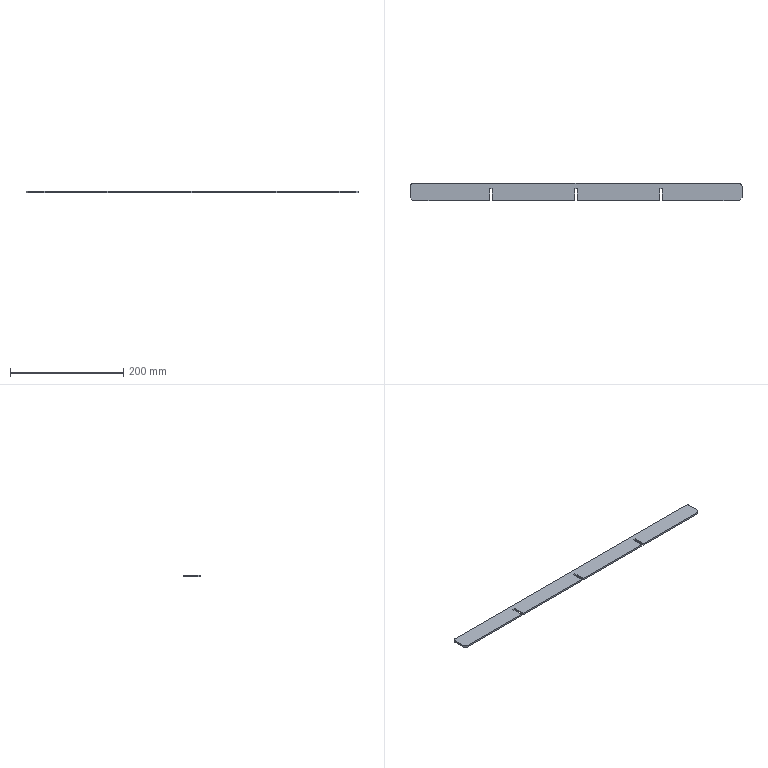Part | SolidWorks | features FlatPattern 1, SMBaseFlange 1, SheetMetal 1 | 1 solid | 22 faces | box 585.4 x 30 x 3 mm | volume 51728 mm3 | plane 20 | cylinder 2 | commonest cylinder face diameters 10 x2
STEP:
#1=CARTESIAN_POINT('',(-293.386,-592.7,0.));
#2=VERTEX_POINT('',#1);
#3=CARTESIAN_POINT('',(-288.386,-597.7,0.));
#4=VERTEX_POINT('',#3);
#5=CARTESIAN_POINT('',(-293.386,-592.7,0.));
#6=DIRECTION('',(0.7071,-0.7071,0.));
#7=VECTOR('',#6,1000.);
#8=LINE('',#5,#7);
#9=EDGE_CURVE('',#2,#4,#8,.T.);
#10=ORIENTED_EDGE('',*,*,#9,.F.);
#11=CARTESIAN_POINT('',(-293.386,-592.7,-3.));
#12=VERTEX_POINT('',#11);
#13=CARTESIAN_POINT('',(-293.386,-592.7,-3.));
#14=DIRECTION('',(0.,0.,1.));
#15=VECTOR('',#14,1000.);
#16=LINE('',#13,#15);
#17=EDGE_CURVE('',#12,#2,#16,.T.);
#18=ORIENTED_EDGE('',*,*,#17,.F.);
#19=CARTESIAN_POINT('',(-288.386,-597.7,-3.));
#20=VERTEX_POINT('',#19);
#21=CARTESIAN_POINT('',(-293.386,-592.7,-3.));
#22=DIRECTION('',(0.7071,-0.7071,0.));
#23=VECTOR('',#22,1000.);
#24=LINE('',#21,#23);
#25=EDGE_CURVE('',#12,#20,#24,.T.);
#26=ORIENTED_EDGE('',*,*,#25,.T.);
#27=CARTESIAN_POINT('',(-288.386,-597.7,-3.));
#28=DIRECTION('',(0.,0.,1.));
#29=VECTOR('',#28,1000.);
#30=LINE('',#27,#29);
#31=EDGE_CURVE('',#20,#4,#30,.T.);
#32=ORIENTED_EDGE('',*,*,#31,.T.);
#33=EDGE_LOOP('',(#10,#18,#26,#32));
#34=FACE_OUTER_BOUND('',#33,.T.);
#35=CARTESIAN_POINT('',(-293.386,-592.7,-3.));
#36=DIRECTION('',(-0.7071,-0.7071,0.));
#37=DIRECTION('',(0.7071,-0.7071,0.));
#38=AXIS2_PLACEMENT_3D('',#35,#36,#37);
#39=PLANE('',#38);
#40=ADVANCED_FACE('',(#34),#39,.T.);
#41=CARTESIAN_POINT('',(-293.386,-572.7,0.));
#42=VERTEX_POINT('',#41);
#43=CARTESIAN_POINT('',(-293.386,-572.7,0.));
#44=DIRECTION('',(0.,-1.,0.));
#45=VECTOR('',#44,1000.);
#46=LINE('',#43,#45);
#47=EDGE_CURVE('',#42,#2,#46,.T.);
#48=ORIENTED_EDGE('',*,*,#47,.F.);
#49=CARTESIAN_POINT('',(-293.386,-572.7,-3.));
#50=VERTEX_POINT('',#49);
#51=CARTESIAN_POINT('',(-293.386,-572.7,-3.));
#52=DIRECTION('',(0.,0.,1.));
#53=VECTOR('',#52,1000.);
#54=LINE('',#51,#53);
#55=EDGE_CURVE('',#50,#42,#54,.T.);
#56=ORIENTED_EDGE('',*,*,#55,.F.);
#57=CARTESIAN_POINT('',(-293.386,-572.7,-3.));
#58=DIRECTION('',(0.,-1.,0.));
#59=VECTOR('',#58,1000.);
#60=LINE('',#57,#59);
#61=EDGE_CURVE('',#50,#12,#60,.T.);
#62=ORIENTED_EDGE('',*,*,#61,.T.);
#63=ORIENTED_EDGE('',*,*,#17,.T.);
#64=EDGE_LOOP('',(#48,#56,#62,#63));
#65=FACE_OUTER_BOUND('',#64,.T.);
#66=CARTESIAN_POINT('',(-293.386,-572.7,-3.));
#67=DIRECTION('',(-1.,0.,0.));
#68=DIRECTION('',(0.,0.,1.));
#69=AXIS2_PLACEMENT_3D('',#66,#67,#68);
#70=PLANE('',#69);
#71=ADVANCED_FACE('',(#65),#70,.T.);
#72=CARTESIAN_POINT('',(-288.386,-567.7,0.));
#73=VERTEX_POINT('',#72);
#74=CARTESIAN_POINT('',(-288.386,-572.7,0.));
#75=DIRECTION('',(0.,0.,1.));
#76=DIRECTION('',(1.,0.,0.));
#77=AXIS2_PLACEMENT_3D('',#74,#75,#76);
#78=CIRCLE('',#77,5.);
#79=EDGE_CURVE('',#73,#42,#78,.T.);
#80=ORIENTED_EDGE('',*,*,#79,.F.);
#81=CARTESIAN_POINT('',(-288.386,-567.7,-3.));
#82=VERTEX_POINT('',#81);
#83=CARTESIAN_POINT('',(-288.386,-567.7,-3.));
#84=DIRECTION('',(0.,0.,1.));
#85=VECTOR('',#84,1000.);
#86=LINE('',#83,#85);
#87=EDGE_CURVE('',#82,#73,#86,.T.);
#88=ORIENTED_EDGE('',*,*,#87,.F.);
#89=CARTESIAN_POINT('',(-288.386,-572.7,-3.));
#90=DIRECTION('',(0.,0.,1.));
#91=DIRECTION('',(1.,0.,0.));
#92=AXIS2_PLACEMENT_3D('',#89,#90,#91);
#93=CIRCLE('',#92,5.);
#94=EDGE_CURVE('',#82,#50,#93,.T.);
#95=ORIENTED_EDGE('',*,*,#94,.T.);
#96=ORIENTED_EDGE('',*,*,#55,.T.);
#97=EDGE_LOOP('',(#80,#88,#95,#96));
#98=FACE_OUTER_BOUND('',#97,.T.);
#99=CARTESIAN_POINT('',(-288.386,-572.7,-3.));
#100=DIRECTION('',(0.,0.,1.));
#101=DIRECTION('',(1.,0.,0.));
#102=AXIS2_PLACEMENT_3D('',#99,#100,#101);
#103=CYLINDRICAL_SURFACE('',#102,5.);
#104=ADVANCED_FACE('',(#98),#103,.T.);
#105=CARTESIAN_POINT('',(287.014,-567.7,0.));
#106=VERTEX_POINT('',#105);
#107=CARTESIAN_POINT('',(287.014,-567.7,0.));
#108=DIRECTION('',(-1.,0.,0.));
#109=VECTOR('',#108,1000.);
#110=LINE('',#107,#109);
#111=EDGE_CURVE('',#106,#73,#110,.T.);
#112=ORIENTED_EDGE('',*,*,#111,.F.);
#113=CARTESIAN_POINT('',(287.014,-567.7,-3.));
#114=VERTEX_POINT('',#113);
#115=CARTESIAN_POINT('',(287.014,-567.7,-3.));
#116=DIRECTION('',(0.,0.,1.));
#117=VECTOR('',#116,1000.);
#118=LINE('',#115,#117);
#119=EDGE_CURVE('',#114,#106,#118,.T.);
#120=ORIENTED_EDGE('',*,*,#119,.F.);
#121=CARTESIAN_POINT('',(287.014,-567.7,-3.));
#122=DIRECTION('',(-1.,0.,0.));
#123=VECTOR('',#122,1000.);
#124=LINE('',#121,#123);
#125=EDGE_CURVE('',#114,#82,#124,.T.);
#126=ORIENTED_EDGE('',*,*,#125,.T.);
#127=ORIENTED_EDGE('',*,*,#87,.T.);
#128=EDGE_LOOP('',(#112,#120,#126,#127));
#129=FACE_OUTER_BOUND('',#128,.T.);
#130=CARTESIAN_POINT('',(287.014,-567.7,-3.));
#131=DIRECTION('',(0.,1.,0.));
#132=DIRECTION('',(-1.,0.,0.));
#133=AXIS2_PLACEMENT_3D('',#130,#131,#132);
#134=PLANE('',#133);
#135=ADVANCED_FACE('',(#129),#134,.T.);
#136=CARTESIAN_POINT('',(292.014,-572.7,0.));
#137=VERTEX_POINT('',#136);
#138=CARTESIAN_POINT('',(287.014,-572.7,0.));
#139=DIRECTION('',(0.,0.,1.));
#140=DIRECTION('',(-1.,0.,0.));
#141=AXIS2_PLACEMENT_3D('',#138,#139,#140);
#142=CIRCLE('',#141,5.);
#143=EDGE_CURVE('',#137,#106,#142,.T.);
#144=ORIENTED_EDGE('',*,*,#143,.F.);
#145=CARTESIAN_POINT('',(292.014,-572.7,-3.));
#146=VERTEX_POINT('',#145);
#147=CARTESIAN_POINT('',(292.014,-572.7,-3.));
#148=DIRECTION('',(0.,0.,1.));
#149=VECTOR('',#148,1000.);
#150=LINE('',#147,#149);
#151=EDGE_CURVE('',#146,#137,#150,.T.);
#152=ORIENTED_EDGE('',*,*,#151,.F.);
#153=CARTESIAN_POINT('',(287.014,-572.7,-3.));
#154=DIRECTION('',(0.,0.,1.));
#155=DIRECTION('',(-1.,0.,0.));
#156=AXIS2_PLACEMENT_3D('',#153,#154,#155);
#157=CIRCLE('',#156,5.);
#158=EDGE_CURVE('',#146,#114,#157,.T.);
#159=ORIENTED_EDGE('',*,*,#158,.T.);
#160=ORIENTED_EDGE('',*,*,#119,.T.);
#161=EDGE_LOOP('',(#144,#152,#159,#160));
#162=FACE_OUTER_BOUND('',#161,.T.);
#163=CARTESIAN_POINT('',(287.014,-572.7,-3.));
#164=DIRECTION('',(0.,0.,1.));
#165=DIRECTION('',(1.,0.,0.));
#166=AXIS2_PLACEMENT_3D('',#163,#164,#165);
#167=CYLINDRICAL_SURFACE('',#166,5.);
#168=ADVANCED_FACE('',(#162),#167,.T.);
#169=CARTESIAN_POINT('',(292.014,-592.7,0.));
#170=VERTEX_POINT('',#169);
#171=CARTESIAN_POINT('',(292.014,-592.7,0.));
#172=DIRECTION('',(0.,1.,0.));
#173=VECTOR('',#172,1000.);
#174=LINE('',#171,#173);
#175=EDGE_CURVE('',#170,#137,#174,.T.);
#176=ORIENTED_EDGE('',*,*,#175,.F.);
#177=CARTESIAN_POINT('',(292.014,-592.7,-3.));
#178=VERTEX_POINT('',#177);
#179=CARTESIAN_POINT('',(292.014,-592.7,-3.));
#180=DIRECTION('',(0.,0.,1.));
#181=VECTOR('',#180,1000.);
#182=LINE('',#179,#181);
#183=EDGE_CURVE('',#178,#170,#182,.T.);
#184=ORIENTED_EDGE('',*,*,#183,.F.);
#185=CARTESIAN_POINT('',(292.014,-592.7,-3.));
#186=DIRECTION('',(0.,1.,0.));
#187=VECTOR('',#186,1000.);
#188=LINE('',#185,#187);
#189=EDGE_CURVE('',#178,#146,#188,.T.);
#190=ORIENTED_EDGE('',*,*,#189,.T.);
#191=ORIENTED_EDGE('',*,*,#151,.T.);
#192=EDGE_LOOP('',(#176,#184,#190,#191));
#193=FACE_OUTER_BOUND('',#192,.T.);
#194=CARTESIAN_POINT('',(292.014,-592.7,-3.));
#195=DIRECTION('',(1.,0.,0.));
#196=DIRECTION('',(0.,0.,-1.));
#197=AXIS2_PLACEMENT_3D('',#194,#195,#196);
#198=PLANE('',#197);
#199=ADVANCED_FACE('',(#193),#198,.T.);
#200=CARTESIAN_POINT('',(287.014,-597.7,0.));
#201=VERTEX_POINT('',#200);
#202=CARTESIAN_POINT('',(287.014,-597.7,0.));
#203=DIRECTION('',(0.7071,0.7071,0.));
#204=VECTOR('',#203,1000.);
#205=LINE('',#202,#204);
#206=EDGE_CURVE('',#201,#170,#205,.T.);
#207=ORIENTED_EDGE('',*,*,#206,.F.);
#208=CARTESIAN_POINT('',(287.014,-597.7,-3.));
#209=VERTEX_POINT('',#208);
#210=CARTESIAN_POINT('',(287.014,-597.7,-3.));
#211=DIRECTION('',(0.,0.,1.));
#212=VECTOR('',#211,1000.);
#213=LINE('',#210,#212);
#214=EDGE_CURVE('',#209,#201,#213,.T.);
#215=ORIENTED_EDGE('',*,*,#214,.F.);
#216=CARTESIAN_POINT('',(287.014,-597.7,-3.));
#217=DIRECTION('',(0.7071,0.7071,0.));
#218=VECTOR('',#217,1000.);
#219=LINE('',#216,#218);
#220=EDGE_CURVE('',#209,#178,#219,.T.);
#221=ORIENTED_EDGE('',*,*,#220,.T.);
#222=ORIENTED_EDGE('',*,*,#183,.T.);
#223=EDGE_LOOP('',(#207,#215,#221,#222));
#224=FACE_OUTER_BOUND('',#223,.T.);
#225=CARTESIAN_POINT('',(287.014,-597.7,-3.));
#226=DIRECTION('',(0.7071,-0.7071,0.));
#227=DIRECTION('',(0.7071,0.7071,0.));
#228=AXIS2_PLACEMENT_3D('',#225,#226,#227);
#229=PLANE('',#228);
#230=ADVANCED_FACE('',(#224),#229,.T.);
#231=CARTESIAN_POINT('',(151.564,-597.7,0.));
#232=VERTEX_POINT('',#231);
#233=CARTESIAN_POINT('',(151.564,-597.7,0.));
#234=DIRECTION('',(1.,0.,0.));
#235=VECTOR('',#234,1000.);
#236=LINE('',#233,#235);
#237=EDGE_CURVE('',#232,#201,#236,.T.);
#238=ORIENTED_EDGE('',*,*,#237,.F.);
#239=CARTESIAN_POINT('',(151.564,-597.7,-3.));
#240=VERTEX_POINT('',#239);
#241=CARTESIAN_POINT('',(151.564,-597.7,-3.));
#242=DIRECTION('',(0.,0.,1.));
#243=VECTOR('',#242,1000.);
#244=LINE('',#241,#243);
#245=EDGE_CURVE('',#240,#232,#244,.T.);
#246=ORIENTED_EDGE('',*,*,#245,.F.);
#247=CARTESIAN_POINT('',(151.564,-597.7,-3.));
#248=DIRECTION('',(1.,0.,0.));
#249=VECTOR('',#248,1000.);
#250=LINE('',#247,#249);
#251=EDGE_CURVE('',#240,#209,#250,.T.);
#252=ORIENTED_EDGE('',*,*,#251,.T.);
#253=ORIENTED_EDGE('',*,*,#214,.T.);
#254=EDGE_LOOP('',(#238,#246,#252,#253));
#255=FACE_OUTER_BOUND('',#254,.T.);
#256=CARTESIAN_POINT('',(151.564,-597.7,-3.));
#257=DIRECTION('',(0.,-1.,0.));
#258=DIRECTION('',(1.,0.,0.));
#259=AXIS2_PLACEMENT_3D('',#256,#257,#258);
#260=PLANE('',#259);
#261=ADVANCED_FACE('',(#255),#260,.T.);
#262=CARTESIAN_POINT('',(151.564,-576.7,0.));
#263=VERTEX_POINT('',#262);
#264=CARTESIAN_POINT('',(151.564,-576.7,0.));
#265=DIRECTION('',(0.,-1.,0.));
#266=VECTOR('',#265,1000.);
#267=LINE('',#264,#266);
#268=EDGE_CURVE('',#263,#232,#267,.T.);
#269=ORIENTED_EDGE('',*,*,#268,.F.);
#270=CARTESIAN_POINT('',(151.564,-576.7,-3.));
#271=VERTEX_POINT('',#270);
#272=CARTESIAN_POINT('',(151.564,-576.7,-3.));
#273=DIRECTION('',(0.,0.,1.));
#274=VECTOR('',#273,1000.);
#275=LINE('',#272,#274);
#276=EDGE_CURVE('',#271,#263,#275,.T.);
#277=ORIENTED_EDGE('',*,*,#276,.F.);
#278=CARTESIAN_POINT('',(151.564,-576.7,-3.));
#279=DIRECTION('',(0.,-1.,0.));
#280=VECTOR('',#279,1000.);
#281=LINE('',#278,#280);
#282=EDGE_CURVE('',#271,#240,#281,.T.);
#283=ORIENTED_EDGE('',*,*,#282,.T.);
#284=ORIENTED_EDGE('',*,*,#245,.T.);
#285=EDGE_LOOP('',(#269,#277,#283,#284));
#286=FACE_OUTER_BOUND('',#285,.T.);
#287=CARTESIAN_POINT('',(151.564,-576.7,-3.));
#288=DIRECTION('',(-1.,0.,0.));
#289=DIRECTION('',(0.,0.,1.));
#290=AXIS2_PLACEMENT_3D('',#287,#288,#289);
#291=PLANE('',#290);
#292=ADVANCED_FACE('',(#286),#291,.T.);
#293=CARTESIAN_POINT('',(147.064,-576.7,0.));
#294=VERTEX_POINT('',#293);
#295=CARTESIAN_POINT('',(147.064,-576.7,0.));
#296=DIRECTION('',(1.,0.,0.));
#297=VECTOR('',#296,1000.);
#298=LINE('',#295,#297);
#299=EDGE_CURVE('',#294,#263,#298,.T.);
#300=ORIENTED_EDGE('',*,*,#299,.F.);
#301=CARTESIAN_POINT('',(147.064,-576.7,-3.));
#302=VERTEX_POINT('',#301);
#303=CARTESIAN_POINT('',(147.064,-576.7,-3.));
#304=DIRECTION('',(0.,0.,1.));
#305=VECTOR('',#304,1000.);
#306=LINE('',#303,#305);
#307=EDGE_CURVE('',#302,#294,#306,.T.);
#308=ORIENTED_EDGE('',*,*,#307,.F.);
#309=CARTESIAN_POINT('',(147.064,-576.7,-3.));
#310=DIRECTION('',(1.,0.,0.));
#311=VECTOR('',#310,1000.);
#312=LINE('',#309,#311);
#313=EDGE_CURVE('',#302,#271,#312,.T.);
#314=ORIENTED_EDGE('',*,*,#313,.T.);
#315=ORIENTED_EDGE('',*,*,#276,.T.);
#316=EDGE_LOOP('',(#300,#308,#314,#315));
#317=FACE_OUTER_BOUND('',#316,.T.);
#318=CARTESIAN_POINT('',(147.064,-576.7,-3.));
#319=DIRECTION('',(0.,-1.,0.));
#320=DIRECTION('',(0.,0.,-1.));
#321=AXIS2_PLACEMENT_3D('',#318,#319,#320);
#322=PLANE('',#321);
#323=ADVANCED_FACE('',(#317),#322,.T.);
#324=CARTESIAN_POINT('',(147.064,-597.7,0.));
#325=VERTEX_POINT('',#324);
#326=CARTESIAN_POINT('',(147.064,-597.7,0.));
#327=DIRECTION('',(0.,1.,0.));
#328=VECTOR('',#327,1000.);
#329=LINE('',#326,#328);
#330=EDGE_CURVE('',#325,#294,#329,.T.);
#331=ORIENTED_EDGE('',*,*,#330,.F.);
#332=CARTESIAN_POINT('',(147.064,-597.7,-3.));
#333=VERTEX_POINT('',#332);
#334=CARTESIAN_POINT('',(147.064,-597.7,-3.));
#335=DIRECTION('',(0.,0.,1.));
#336=VECTOR('',#335,1000.);
#337=LINE('',#334,#336);
#338=EDGE_CURVE('',#333,#325,#337,.T.);
#339=ORIENTED_EDGE('',*,*,#338,.F.);
#340=CARTESIAN_POINT('',(147.064,-597.7,-3.));
#341=DIRECTION('',(0.,1.,0.));
#342=VECTOR('',#341,1000.);
#343=LINE('',#340,#342);
#344=EDGE_CURVE('',#333,#302,#343,.T.);
#345=ORIENTED_EDGE('',*,*,#344,.T.);
#346=ORIENTED_EDGE('',*,*,#307,.T.);
#347=EDGE_LOOP('',(#331,#339,#345,#346));
#348=FACE_OUTER_BOUND('',#347,.T.);
#349=CARTESIAN_POINT('',(147.064,-597.7,-3.));
#350=DIRECTION('',(1.,0.,0.));
#351=DIRECTION('',(0.,0.,-1.));
#352=AXIS2_PLACEMENT_3D('',#349,#350,#351);
#353=PLANE('',#352);
#354=ADVANCED_FACE('',(#348),#353,.T.);
#355=CARTESIAN_POINT('',(1.564,-597.7,0.));
#356=VERTEX_POINT('',#355);
#357=CARTESIAN_POINT('',(1.564,-597.7,0.));
#358=DIRECTION('',(1.,0.,0.));
#359=VECTOR('',#358,1000.);
#360=LINE('',#357,#359);
#361=EDGE_CURVE('',#356,#325,#360,.T.);
#362=ORIENTED_EDGE('',*,*,#361,.F.);
#363=CARTESIAN_POINT('',(1.564,-597.7,-3.));
#364=VERTEX_POINT('',#363);
#365=CARTESIAN_POINT('',(1.564,-597.7,-3.));
#366=DIRECTION('',(0.,0.,1.));
#367=VECTOR('',#366,1000.);
#368=LINE('',#365,#367);
#369=EDGE_CURVE('',#364,#356,#368,.T.);
#370=ORIENTED_EDGE('',*,*,#369,.F.);
#371=CARTESIAN_POINT('',(1.564,-597.7,-3.));
#372=DIRECTION('',(1.,0.,0.));
#373=VECTOR('',#372,1000.);
#374=LINE('',#371,#373);
#375=EDGE_CURVE('',#364,#333,#374,.T.);
#376=ORIENTED_EDGE('',*,*,#375,.T.);
#377=ORIENTED_EDGE('',*,*,#338,.T.);
#378=EDGE_LOOP('',(#362,#370,#376,#377));
#379=FACE_OUTER_BOUND('',#378,.T.);
#380=CARTESIAN_POINT('',(1.564,-597.7,-3.));
#381=DIRECTION('',(0.,-1.,0.));
#382=DIRECTION('',(1.,0.,0.));
#383=AXIS2_PLACEMENT_3D('',#380,#381,#382);
#384=PLANE('',#383);
#385=ADVANCED_FACE('',(#379),#384,.T.);
#386=CARTESIAN_POINT('',(1.564,-576.7,0.));
#387=VERTEX_POINT('',#386);
#388=CARTESIAN_POINT('',(1.564,-576.7,0.));
#389=DIRECTION('',(0.,-1.,0.));
#390=VECTOR('',#389,1000.);
#391=LINE('',#388,#390);
#392=EDGE_CURVE('',#387,#356,#391,.T.);
#393=ORIENTED_EDGE('',*,*,#392,.F.);
#394=CARTESIAN_POINT('',(1.564,-576.7,-3.));
#395=VERTEX_POINT('',#394);
#396=CARTESIAN_POINT('',(1.564,-576.7,-3.));
#397=DIRECTION('',(0.,0.,1.));
#398=VECTOR('',#397,1000.);
#399=LINE('',#396,#398);
#400=EDGE_CURVE('',#395,#387,#399,.T.);
#401=ORIENTED_EDGE('',*,*,#400,.F.);
#402=CARTESIAN_POINT('',(1.564,-576.7,-3.));
#403=DIRECTION('',(0.,-1.,0.));
#404=VECTOR('',#403,1000.);
#405=LINE('',#402,#404);
#406=EDGE_CURVE('',#395,#364,#405,.T.);
#407=ORIENTED_EDGE('',*,*,#406,.T.);
#408=ORIENTED_EDGE('',*,*,#369,.T.);
#409=EDGE_LOOP('',(#393,#401,#407,#408));
#410=FACE_OUTER_BOUND('',#409,.T.);
#411=CARTESIAN_POINT('',(1.564,-576.7,-3.));
#412=DIRECTION('',(-1.,0.,0.));
#413=DIRECTION('',(0.,-1.,0.));
#414=AXIS2_PLACEMENT_3D('',#411,#412,#413);
#415=PLANE('',#414);
#416=ADVANCED_FACE('',(#410),#415,.T.);
#417=CARTESIAN_POINT('',(-2.936,-576.7,0.));
#418=VERTEX_POINT('',#417);
#419=CARTESIAN_POINT('',(-2.936,-576.7,0.));
#420=DIRECTION('',(1.,0.,0.));
#421=VECTOR('',#420,1000.);
#422=LINE('',#419,#421);
#423=EDGE_CURVE('',#418,#387,#422,.T.);
#424=ORIENTED_EDGE('',*,*,#423,.F.);
#425=CARTESIAN_POINT('',(-2.936,-576.7,-3.));
#426=VERTEX_POINT('',#425);
#427=CARTESIAN_POINT('',(-2.936,-576.7,-3.));
#428=DIRECTION('',(0.,0.,1.));
#429=VECTOR('',#428,1000.);
#430=LINE('',#427,#429);
#431=EDGE_CURVE('',#426,#418,#430,.T.);
#432=ORIENTED_EDGE('',*,*,#431,.F.);
#433=CARTESIAN_POINT('',(-2.936,-576.7,-3.));
#434=DIRECTION('',(1.,0.,0.));
#435=VECTOR('',#434,1000.);
#436=LINE('',#433,#435);
#437=EDGE_CURVE('',#426,#395,#436,.T.);
#438=ORIENTED_EDGE('',*,*,#437,.T.);
#439=ORIENTED_EDGE('',*,*,#400,.T.);
#440=EDGE_LOOP('',(#424,#432,#438,#439));
#441=FACE_OUTER_BOUND('',#440,.T.);
#442=CARTESIAN_POINT('',(-2.936,-576.7,-3.));
#443=DIRECTION('',(0.,-1.,0.));
#444=DIRECTION('',(0.,0.,-1.));
#445=AXIS2_PLACEMENT_3D('',#442,#443,#444);
#446=PLANE('',#445);
#447=ADVANCED_FACE('',(#441),#446,.T.);
#448=CARTESIAN_POINT('',(-2.936,-597.7,0.));
#449=VERTEX_POINT('',#448);
#450=CARTESIAN_POINT('',(-2.936,-597.7,0.));
#451=DIRECTION('',(0.,1.,0.));
#452=VECTOR('',#451,1000.);
#453=LINE('',#450,#452);
#454=EDGE_CURVE('',#449,#418,#453,.T.);
#455=ORIENTED_EDGE('',*,*,#454,.F.);
#456=CARTESIAN_POINT('',(-2.936,-597.7,-3.));
#457=VERTEX_POINT('',#456);
#458=CARTESIAN_POINT('',(-2.936,-597.7,-3.));
#459=DIRECTION('',(0.,0.,1.));
#460=VECTOR('',#459,1000.);
#461=LINE('',#458,#460);
#462=EDGE_CURVE('',#457,#449,#461,.T.);
#463=ORIENTED_EDGE('',*,*,#462,.F.);
#464=CARTESIAN_POINT('',(-2.936,-597.7,-3.));
#465=DIRECTION('',(0.,1.,0.));
#466=VECTOR('',#465,1000.);
#467=LINE('',#464,#466);
#468=EDGE_CURVE('',#457,#426,#467,.T.);
#469=ORIENTED_EDGE('',*,*,#468,.T.);
#470=ORIENTED_EDGE('',*,*,#431,.T.);
#471=EDGE_LOOP('',(#455,#463,#469,#470));
#472=FACE_OUTER_BOUND('',#471,.T.);
#473=CARTESIAN_POINT('',(-2.936,-597.7,-3.));
#474=DIRECTION('',(1.,0.,0.));
#475=DIRECTION('',(0.,0.,-1.));
#476=AXIS2_PLACEMENT_3D('',#473,#474,#475);
#477=PLANE('',#476);
#478=ADVANCED_FACE('',(#472),#477,.T.);
#479=CARTESIAN_POINT('',(-148.436,-597.7,0.));
#480=VERTEX_POINT('',#479);
#481=CARTESIAN_POINT('',(-148.436,-597.7,0.));
#482=DIRECTION('',(1.,0.,0.));
#483=VECTOR('',#482,1000.);
#484=LINE('',#481,#483);
#485=EDGE_CURVE('',#480,#449,#484,.T.);
#486=ORIENTED_EDGE('',*,*,#485,.F.);
#487=CARTESIAN_POINT('',(-148.436,-597.7,-3.));
#488=VERTEX_POINT('',#487);
#489=CARTESIAN_POINT('',(-148.436,-597.7,-3.));
#490=DIRECTION('',(0.,0.,1.));
#491=VECTOR('',#490,1000.);
#492=LINE('',#489,#491);
#493=EDGE_CURVE('',#488,#480,#492,.T.);
#494=ORIENTED_EDGE('',*,*,#493,.F.);
#495=CARTESIAN_POINT('',(-148.436,-597.7,-3.));
#496=DIRECTION('',(1.,0.,0.));
#497=VECTOR('',#496,1000.);
#498=LINE('',#495,#497);
#499=EDGE_CURVE('',#488,#457,#498,.T.);
#500=ORIENTED_EDGE('',*,*,#499,.T.);
#501=ORIENTED_EDGE('',*,*,#462,.T.);
#502=EDGE_LOOP('',(#486,#494,#500,#501));
#503=FACE_OUTER_BOUND('',#502,.T.);
#504=CARTESIAN_POINT('',(-148.436,-597.7,-3.));
#505=DIRECTION('',(0.,-1.,0.));
#506=DIRECTION('',(1.,0.,0.));
#507=AXIS2_PLACEMENT_3D('',#504,#505,#506);
#508=PLANE('',#507);
#509=ADVANCED_FACE('',(#503),#508,.T.);
#510=CARTESIAN_POINT('',(-148.436,-576.7,0.));
#511=VERTEX_POINT('',#510);
#512=CARTESIAN_POINT('',(-148.436,-576.7,0.));
#513=DIRECTION('',(0.,-1.,0.));
#514=VECTOR('',#513,1000.);
#515=LINE('',#512,#514);
#516=EDGE_CURVE('',#511,#480,#515,.T.);
#517=ORIENTED_EDGE('',*,*,#516,.F.);
#518=CARTESIAN_POINT('',(-148.436,-576.7,-3.));
#519=VERTEX_POINT('',#518);
#520=CARTESIAN_POINT('',(-148.436,-576.7,-3.));
#521=DIRECTION('',(0.,0.,1.));
#522=VECTOR('',#521,1000.);
#523=LINE('',#520,#522);
#524=EDGE_CURVE('',#519,#511,#523,.T.);
#525=ORIENTED_EDGE('',*,*,#524,.F.);
#526=CARTESIAN_POINT('',(-148.436,-576.7,-3.));
#527=DIRECTION('',(0.,-1.,0.));
#528=VECTOR('',#527,1000.);
#529=LINE('',#526,#528);
#530=EDGE_CURVE('',#519,#488,#529,.T.);
#531=ORIENTED_EDGE('',*,*,#530,.T.);
#532=ORIENTED_EDGE('',*,*,#493,.T.);
#533=EDGE_LOOP('',(#517,#525,#531,#532));
#534=FACE_OUTER_BOUND('',#533,.T.);
#535=CARTESIAN_POINT('',(-148.436,-576.7,-3.));
#536=DIRECTION('',(-1.,0.,0.));
#537=DIRECTION('',(0.,0.,1.));
#538=AXIS2_PLACEMENT_3D('',#535,#536,#537);
#539=PLANE('',#538);
#540=ADVANCED_FACE('',(#534),#539,.T.);
#541=CARTESIAN_POINT('',(-152.936,-576.7,0.));
#542=VERTEX_POINT('',#541);
#543=CARTESIAN_POINT('',(-152.936,-576.7,0.));
#544=DIRECTION('',(1.,0.,0.));
#545=VECTOR('',#544,1000.);
#546=LINE('',#543,#545);
#547=EDGE_CURVE('',#542,#511,#546,.T.);
#548=ORIENTED_EDGE('',*,*,#547,.F.);
#549=CARTESIAN_POINT('',(-152.936,-576.7,-3.));
#550=VERTEX_POINT('',#549);
#551=CARTESIAN_POINT('',(-152.936,-576.7,-3.));
#552=DIRECTION('',(0.,0.,1.));
#553=VECTOR('',#552,1000.);
#554=LINE('',#551,#553);
#555=EDGE_CURVE('',#550,#542,#554,.T.);
#556=ORIENTED_EDGE('',*,*,#555,.F.);
#557=CARTESIAN_POINT('',(-152.936,-576.7,-3.));
#558=DIRECTION('',(1.,0.,0.));
#559=VECTOR('',#558,1000.);
#560=LINE('',#557,#559);
#561=EDGE_CURVE('',#550,#519,#560,.T.);
#562=ORIENTED_EDGE('',*,*,#561,.T.);
#563=ORIENTED_EDGE('',*,*,#524,.T.);
#564=EDGE_LOOP('',(#548,#556,#562,#563));
#565=FACE_OUTER_BOUND('',#564,.T.);
#566=CARTESIAN_POINT('',(-152.936,-576.7,-3.));
#567=DIRECTION('',(0.,-1.,0.));
#568=DIRECTION('',(0.,0.,-1.));
#569=AXIS2_PLACEMENT_3D('',#566,#567,#568);
#570=PLANE('',#569);
#571=ADVANCED_FACE('',(#565),#570,.T.);
#572=CARTESIAN_POINT('',(-152.936,-597.7,0.));
#573=VERTEX_POINT('',#572);
#574=CARTESIAN_POINT('',(-152.936,-597.7,0.));
#575=DIRECTION('',(0.,1.,0.));
#576=VECTOR('',#575,1000.);
#577=LINE('',#574,#576);
#578=EDGE_CURVE('',#573,#542,#577,.T.);
#579=ORIENTED_EDGE('',*,*,#578,.F.);
#580=CARTESIAN_POINT('',(-152.936,-597.7,-3.));
#581=VERTEX_POINT('',#580);
#582=CARTESIAN_POINT('',(-152.936,-597.7,-3.));
#583=DIRECTION('',(0.,0.,1.));
#584=VECTOR('',#583,1000.);
#585=LINE('',#582,#584);
#586=EDGE_CURVE('',#581,#573,#585,.T.);
#587=ORIENTED_EDGE('',*,*,#586,.F.);
#588=CARTESIAN_POINT('',(-152.936,-597.7,-3.));
#589=DIRECTION('',(0.,1.,0.));
#590=VECTOR('',#589,1000.);
#591=LINE('',#588,#590);
#592=EDGE_CURVE('',#581,#550,#591,.T.);
#593=ORIENTED_EDGE('',*,*,#592,.T.);
#594=ORIENTED_EDGE('',*,*,#555,.T.);
#595=EDGE_LOOP('',(#579,#587,#593,#594));
#596=FACE_OUTER_BOUND('',#595,.T.);
#597=CARTESIAN_POINT('',(-152.936,-597.7,-3.));
#598=DIRECTION('',(1.,0.,0.));
#599=DIRECTION('',(0.,0.,-1.));
#600=AXIS2_PLACEMENT_3D('',#597,#598,#599);
#601=PLANE('',#600);
#602=ADVANCED_FACE('',(#596),#601,.T.);
#603=CARTESIAN_POINT('',(-288.386,-597.7,0.));
#604=DIRECTION('',(1.,0.,0.));
#605=VECTOR('',#604,1000.);
#606=LINE('',#603,#605);
#607=EDGE_CURVE('',#4,#573,#606,.T.);
#608=ORIENTED_EDGE('',*,*,#607,.F.);
#609=ORIENTED_EDGE('',*,*,#31,.F.);
#610=CARTESIAN_POINT('',(-288.386,-597.7,-3.));
#611=DIRECTION('',(1.,0.,0.));
#612=VECTOR('',#611,1000.);
#613=LINE('',#610,#612);
#614=EDGE_CURVE('',#20,#581,#613,.T.);
#615=ORIENTED_EDGE('',*,*,#614,.T.);
#616=ORIENTED_EDGE('',*,*,#586,.T.);
#617=EDGE_LOOP('',(#608,#609,#615,#616));
#618=FACE_OUTER_BOUND('',#617,.T.);
#619=CARTESIAN_POINT('',(-288.386,-597.7,-3.));
#620=DIRECTION('',(0.,-1.,0.));
#621=DIRECTION('',(1.,0.,0.));
#622=AXIS2_PLACEMENT_3D('',#619,#620,#621);
#623=PLANE('',#622);
#624=ADVANCED_FACE('',(#618),#623,.T.);
#625=ORIENTED_EDGE('',*,*,#25,.F.);
#626=ORIENTED_EDGE('',*,*,#61,.F.);
#627=ORIENTED_EDGE('',*,*,#94,.F.);
#628=ORIENTED_EDGE('',*,*,#125,.F.);
#629=ORIENTED_EDGE('',*,*,#158,.F.);
#630=ORIENTED_EDGE('',*,*,#189,.F.);
#631=ORIENTED_EDGE('',*,*,#220,.F.);
#632=ORIENTED_EDGE('',*,*,#251,.F.);
#633=ORIENTED_EDGE('',*,*,#282,.F.);
#634=ORIENTED_EDGE('',*,*,#313,.F.);
#635=ORIENTED_EDGE('',*,*,#344,.F.);
#636=ORIENTED_EDGE('',*,*,#375,.F.);
#637=ORIENTED_EDGE('',*,*,#406,.F.);
#638=ORIENTED_EDGE('',*,*,#437,.F.);
#639=ORIENTED_EDGE('',*,*,#468,.F.);
#640=ORIENTED_EDGE('',*,*,#499,.F.);
#641=ORIENTED_EDGE('',*,*,#530,.F.);
#642=ORIENTED_EDGE('',*,*,#561,.F.);
#643=ORIENTED_EDGE('',*,*,#592,.F.);
#644=ORIENTED_EDGE('',*,*,#614,.F.);
#645=EDGE_LOOP('',(#625,#626,#627,#628,#629,#630,#631,#632,#633,#634,#635,#636,#637,#638,#639,#640,#641,#642,#643,#644));
#646=FACE_OUTER_BOUND('',#645,.T.);
#647=CARTESIAN_POINT('',(287.014,-572.7,-3.));
#648=DIRECTION('',(0.,0.,-1.));
#649=DIRECTION('',(-1.,0.,0.));
#650=AXIS2_PLACEMENT_3D('',#647,#648,#649);
#651=PLANE('',#650);
#652=ADVANCED_FACE('',(#646),#651,.T.);
#653=ORIENTED_EDGE('',*,*,#9,.T.);
#654=ORIENTED_EDGE('',*,*,#607,.T.);
#655=ORIENTED_EDGE('',*,*,#578,.T.);
#656=ORIENTED_EDGE('',*,*,#547,.T.);
#657=ORIENTED_EDGE('',*,*,#516,.T.);
#658=ORIENTED_EDGE('',*,*,#485,.T.);
#659=ORIENTED_EDGE('',*,*,#454,.T.);
#660=ORIENTED_EDGE('',*,*,#423,.T.);
#661=ORIENTED_EDGE('',*,*,#392,.T.);
#662=ORIENTED_EDGE('',*,*,#361,.T.);
#663=ORIENTED_EDGE('',*,*,#330,.T.);
#664=ORIENTED_EDGE('',*,*,#299,.T.);
#665=ORIENTED_EDGE('',*,*,#268,.T.);
#666=ORIENTED_EDGE('',*,*,#237,.T.);
#667=ORIENTED_EDGE('',*,*,#206,.T.);
#668=ORIENTED_EDGE('',*,*,#175,.T.);
#669=ORIENTED_EDGE('',*,*,#143,.T.);
#670=ORIENTED_EDGE('',*,*,#111,.T.);
#671=ORIENTED_EDGE('',*,*,#79,.T.);
#672=ORIENTED_EDGE('',*,*,#47,.T.);
#673=EDGE_LOOP('',(#653,#654,#655,#656,#657,#658,#659,#660,#661,#662,#663,#664,#665,#666,#667,#668,#669,#670,#671,#672));
#674=FACE_OUTER_BOUND('',#673,.T.);
#675=CARTESIAN_POINT('',(287.014,-572.7,0.));
#676=DIRECTION('',(0.,0.,-1.));
#677=DIRECTION('',(-1.,0.,0.));
#678=AXIS2_PLACEMENT_3D('',#675,#676,#677);
#679=PLANE('',#678);
#680=ADVANCED_FACE('',(#674),#679,.F.);
#681=CLOSED_SHELL('',(#40,#71,#104,#135,#168,#199,#230,#261,#292,#323,#354,#385,#416,#447,#478,#509,#540,#571,#602,#624,#652,#680));
#682=MANIFOLD_SOLID_BREP('',#681);
#683=CARTESIAN_POINT('',(0.,0.,0.));
#684=DIRECTION('',(0.,0.,1.));
#685=DIRECTION('',(1.,0.,0.));
#686=AXIS2_PLACEMENT_3D('',#683,#684,#685);
#687=(LENGTH_UNIT()NAMED_UNIT(*)SI_UNIT(.MILLI.,.METRE.));
#688=UNCERTAINTY_MEASURE_WITH_UNIT(LENGTH_MEASURE(0.00001),#687,'','');
#689=(NAMED_UNIT(*)PLANE_ANGLE_UNIT()SI_UNIT($,.RADIAN.));
#690=(NAMED_UNIT(*)SI_UNIT($,.STERADIAN.)SOLID_ANGLE_UNIT());
#691=(GEOMETRIC_REPRESENTATION_CONTEXT(3)GLOBAL_UNCERTAINTY_ASSIGNED_CONTEXT((#688))GLOBAL_UNIT_ASSIGNED_CONTEXT((#687,#689,#690))REPRESENTATION_CONTEXT('',''));
#692=ADVANCED_BREP_SHAPE_REPRESENTATION('',(#682,#686),#691);